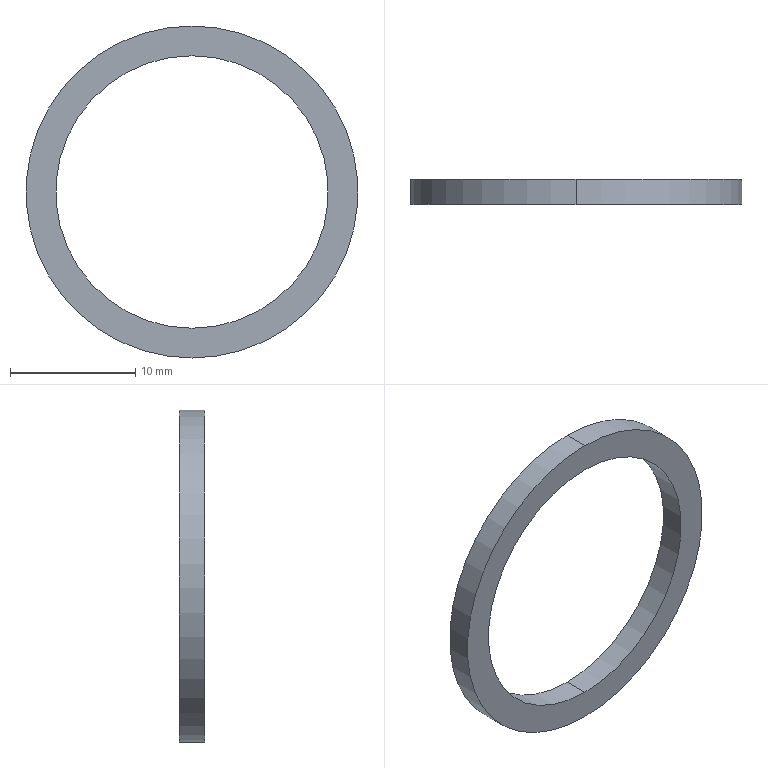Part | STEP file | 00649788_SCHEIBE_MKRT-23-16.5 | 1 solid | 6 faces | box 26.5 x 2 x 26.5 mm | volume 360.007 mm3 | cylinder 4 | plane 2 | commonest cylinder face diameters 21.75 x2 26.5 x2
STEP:
#1=CARTESIAN_POINT('',(0.,0.,0.));
#2=DIRECTION('',(0.,0.,1.));
#3=DIRECTION('',(1.,0.,0.));
#4=AXIS2_PLACEMENT_3D('',#1,#2,#3);
#5=CARTESIAN_POINT('',(0.,43.,10.875));
#6=VERTEX_POINT('',#5);
#7=CARTESIAN_POINT('',(0.,45.,10.875));
#8=VERTEX_POINT('',#7);
#9=CARTESIAN_POINT('',(0.,43.,10.875));
#10=DIRECTION('',(0.,1.,0.));
#11=VECTOR('',#10,1.);
#12=LINE('',#9,#11);
#13=CARTESIAN_POINT('',(0.,43.,0.));
#14=DIRECTION('',(0.,1.,0.));
#15=DIRECTION('',(0.,0.,1.));
#16=AXIS2_PLACEMENT_3D('',#13,#14,#15);
#17=CYLINDRICAL_SURFACE('',#16,10.875);
#18=CARTESIAN_POINT('',(6.283,0.));
#19=DIRECTION('',(0.,1.));
#20=VECTOR('',#19,1.);
#21=LINE('',#18,#20);
#22=(GEOMETRIC_REPRESENTATION_CONTEXT(2)PARAMETRIC_REPRESENTATION_CONTEXT()REPRESENTATION_CONTEXT('',''));
#23=DEFINITIONAL_REPRESENTATION('',(#21),#22);
#24=PCURVE('',#17,#23);
#25=CARTESIAN_POINT('',(0.,43.,0.));
#26=DIRECTION('',(0.,1.,0.));
#27=DIRECTION('',(0.,0.,1.));
#28=AXIS2_PLACEMENT_3D('',#25,#26,#27);
#29=CYLINDRICAL_SURFACE('',#28,10.875);
#30=CARTESIAN_POINT('',(0.,0.));
#31=DIRECTION('',(0.,1.));
#32=VECTOR('',#31,1.);
#33=LINE('',#30,#32);
#34=(GEOMETRIC_REPRESENTATION_CONTEXT(2)PARAMETRIC_REPRESENTATION_CONTEXT()REPRESENTATION_CONTEXT('',''));
#35=DEFINITIONAL_REPRESENTATION('',(#33),#34);
#36=PCURVE('',#29,#35);
#37=SURFACE_CURVE('',#12,(#24,#36),.PCURVE_S1.);
#38=EDGE_CURVE('',#6,#8,#37,.T.);
#39=ORIENTED_EDGE('',*,*,#38,.T.);
#40=CARTESIAN_POINT('',(0.,45.,-10.875));
#41=VERTEX_POINT('',#40);
#42=CARTESIAN_POINT('',(0.,45.,0.));
#43=DIRECTION('',(0.,-1.,0.));
#44=DIRECTION('',(0.,0.,1.));
#45=AXIS2_PLACEMENT_3D('',#42,#43,#44);
#46=CIRCLE('',#45,10.875);
#47=CARTESIAN_POINT('',(6.283,2.));
#48=DIRECTION('',(-1.,0.));
#49=VECTOR('',#48,1.);
#50=LINE('',#47,#49);
#51=(GEOMETRIC_REPRESENTATION_CONTEXT(2)PARAMETRIC_REPRESENTATION_CONTEXT()REPRESENTATION_CONTEXT('',''));
#52=DEFINITIONAL_REPRESENTATION('',(#50),#51);
#53=PCURVE('',#17,#52);
#54=CARTESIAN_POINT('',(40.672,45.,-24.269));
#55=DIRECTION('',(0.,1.,0.));
#56=DIRECTION('',(0.,0.,1.));
#57=AXIS2_PLACEMENT_3D('',#54,#55,#56);
#58=PLANE('',#57);
#59=CARTESIAN_POINT('',(35.144,-40.672));
#60=CARTESIAN_POINT('',(35.144,-59.508));
#61=CARTESIAN_POINT('',(18.831,-50.09));
#62=CARTESIAN_POINT('',(2.519,-40.672));
#63=CARTESIAN_POINT('',(18.831,-31.254));
#64=CARTESIAN_POINT('',(35.144,-21.836));
#65=CARTESIAN_POINT('',(35.144,-40.672));
#66=(BOUNDED_CURVE()B_SPLINE_CURVE(2,(#59,#60,#61,#62,#63,#64,#65),.UNSPECIFIED.,.T.,.F.)B_SPLINE_CURVE_WITH_KNOTS((1,2,2,2,2,1),(-2.094,0.,2.094,4.189,6.283,8.378),.UNSPECIFIED.)CURVE()GEOMETRIC_REPRESENTATION_ITEM()RATIONAL_B_SPLINE_CURVE((1.,0.5,1.,0.5,1.,0.5,1.))REPRESENTATION_ITEM(''));
#67=(GEOMETRIC_REPRESENTATION_CONTEXT(2)PARAMETRIC_REPRESENTATION_CONTEXT()REPRESENTATION_CONTEXT('',''));
#68=DEFINITIONAL_REPRESENTATION('',(#66),#67);
#69=PCURVE('',#58,#68);
#70=SURFACE_CURVE('',#46,(#53,#69),.PCURVE_S1.);
#71=EDGE_CURVE('',#8,#41,#70,.T.);
#72=ORIENTED_EDGE('',*,*,#71,.T.);
#73=CARTESIAN_POINT('',(0.,43.,-10.875));
#74=VERTEX_POINT('',#73);
#75=CARTESIAN_POINT('',(0.,43.,-10.875));
#76=DIRECTION('',(0.,1.,0.));
#77=VECTOR('',#76,1.);
#78=LINE('',#75,#77);
#79=CARTESIAN_POINT('',(3.142,0.));
#80=DIRECTION('',(0.,1.));
#81=VECTOR('',#80,1.);
#82=LINE('',#79,#81);
#83=(GEOMETRIC_REPRESENTATION_CONTEXT(2)PARAMETRIC_REPRESENTATION_CONTEXT()REPRESENTATION_CONTEXT('',''));
#84=DEFINITIONAL_REPRESENTATION('',(#82),#83);
#85=PCURVE('',#17,#84);
#86=CARTESIAN_POINT('',(3.142,0.));
#87=DIRECTION('',(0.,1.));
#88=VECTOR('',#87,1.);
#89=LINE('',#86,#88);
#90=(GEOMETRIC_REPRESENTATION_CONTEXT(2)PARAMETRIC_REPRESENTATION_CONTEXT()REPRESENTATION_CONTEXT('',''));
#91=DEFINITIONAL_REPRESENTATION('',(#89),#90);
#92=PCURVE('',#29,#91);
#93=SURFACE_CURVE('',#78,(#85,#92),.PCURVE_S1.);
#94=EDGE_CURVE('',#74,#41,#93,.T.);
#95=ORIENTED_EDGE('',*,*,#94,.F.);
#96=CARTESIAN_POINT('',(0.,43.,0.));
#97=DIRECTION('',(0.,-1.,0.));
#98=DIRECTION('',(0.,0.,1.));
#99=AXIS2_PLACEMENT_3D('',#96,#97,#98);
#100=CIRCLE('',#99,10.875);
#101=CARTESIAN_POINT('',(6.283,0.));
#102=DIRECTION('',(-1.,0.));
#103=VECTOR('',#102,1.);
#104=LINE('',#101,#103);
#105=(GEOMETRIC_REPRESENTATION_CONTEXT(2)PARAMETRIC_REPRESENTATION_CONTEXT()REPRESENTATION_CONTEXT('',''));
#106=DEFINITIONAL_REPRESENTATION('',(#104),#105);
#107=PCURVE('',#17,#106);
#108=CARTESIAN_POINT('',(40.672,43.,-24.269));
#109=DIRECTION('',(0.,1.,0.));
#110=DIRECTION('',(0.,0.,1.));
#111=AXIS2_PLACEMENT_3D('',#108,#109,#110);
#112=PLANE('',#111);
#113=CARTESIAN_POINT('',(35.144,-40.672));
#114=CARTESIAN_POINT('',(35.144,-59.508));
#115=CARTESIAN_POINT('',(18.831,-50.09));
#116=CARTESIAN_POINT('',(2.519,-40.672));
#117=CARTESIAN_POINT('',(18.831,-31.254));
#118=CARTESIAN_POINT('',(35.144,-21.836));
#119=CARTESIAN_POINT('',(35.144,-40.672));
#120=(BOUNDED_CURVE()B_SPLINE_CURVE(2,(#113,#114,#115,#116,#117,#118,#119),.UNSPECIFIED.,.T.,.F.)B_SPLINE_CURVE_WITH_KNOTS((1,2,2,2,2,1),(-2.094,0.,2.094,4.189,6.283,8.378),.UNSPECIFIED.)CURVE()GEOMETRIC_REPRESENTATION_ITEM()RATIONAL_B_SPLINE_CURVE((1.,0.5,1.,0.5,1.,0.5,1.))REPRESENTATION_ITEM(''));
#121=(GEOMETRIC_REPRESENTATION_CONTEXT(2)PARAMETRIC_REPRESENTATION_CONTEXT()REPRESENTATION_CONTEXT('',''));
#122=DEFINITIONAL_REPRESENTATION('',(#120),#121);
#123=PCURVE('',#112,#122);
#124=SURFACE_CURVE('',#100,(#107,#123),.PCURVE_S1.);
#125=EDGE_CURVE('',#6,#74,#124,.T.);
#126=ORIENTED_EDGE('',*,*,#125,.F.);
#127=EDGE_LOOP('',(#39,#72,#95,#126));
#128=FACE_BOUND('',#127,.F.);
#129=ADVANCED_FACE('',(#128),#17,.F.);
#130=CARTESIAN_POINT('',(0.,43.,13.25));
#131=VERTEX_POINT('',#130);
#132=CARTESIAN_POINT('',(0.,43.,-13.25));
#133=VERTEX_POINT('',#132);
#134=CARTESIAN_POINT('',(0.,43.,0.));
#135=DIRECTION('',(0.,1.,0.));
#136=DIRECTION('',(0.,0.,1.));
#137=AXIS2_PLACEMENT_3D('',#134,#135,#136);
#138=CIRCLE('',#137,13.25);
#139=CARTESIAN_POINT('',(0.,43.,0.));
#140=DIRECTION('',(0.,1.,0.));
#141=DIRECTION('',(0.,0.,1.));
#142=AXIS2_PLACEMENT_3D('',#139,#140,#141);
#143=CYLINDRICAL_SURFACE('',#142,13.25);
#144=CARTESIAN_POINT('',(0.,0.));
#145=DIRECTION('',(1.,0.));
#146=VECTOR('',#145,1.);
#147=LINE('',#144,#146);
#148=(GEOMETRIC_REPRESENTATION_CONTEXT(2)PARAMETRIC_REPRESENTATION_CONTEXT()REPRESENTATION_CONTEXT('',''));
#149=DEFINITIONAL_REPRESENTATION('',(#147),#148);
#150=PCURVE('',#143,#149);
#151=CARTESIAN_POINT('',(24.269,-40.672));
#152=DIRECTION('',(1.,0.));
#153=AXIS2_PLACEMENT_2D('',#151,#152);
#154=CIRCLE('',#153,13.25);
#155=(GEOMETRIC_REPRESENTATION_CONTEXT(2)PARAMETRIC_REPRESENTATION_CONTEXT()REPRESENTATION_CONTEXT('',''));
#156=DEFINITIONAL_REPRESENTATION('',(#154),#155);
#157=PCURVE('',#112,#156);
#158=SURFACE_CURVE('',#138,(#150,#157),.PCURVE_S1.);
#159=EDGE_CURVE('',#131,#133,#158,.T.);
#160=ORIENTED_EDGE('',*,*,#159,.T.);
#161=CARTESIAN_POINT('',(0.,45.,-13.25));
#162=VERTEX_POINT('',#161);
#163=CARTESIAN_POINT('',(0.,43.,-13.25));
#164=DIRECTION('',(0.,1.,0.));
#165=VECTOR('',#164,1.);
#166=LINE('',#163,#165);
#167=CARTESIAN_POINT('',(3.142,0.));
#168=DIRECTION('',(0.,1.));
#169=VECTOR('',#168,1.);
#170=LINE('',#167,#169);
#171=(GEOMETRIC_REPRESENTATION_CONTEXT(2)PARAMETRIC_REPRESENTATION_CONTEXT()REPRESENTATION_CONTEXT('',''));
#172=DEFINITIONAL_REPRESENTATION('',(#170),#171);
#173=PCURVE('',#143,#172);
#174=CARTESIAN_POINT('',(0.,43.,0.));
#175=DIRECTION('',(0.,1.,0.));
#176=DIRECTION('',(0.,0.,1.));
#177=AXIS2_PLACEMENT_3D('',#174,#175,#176);
#178=CYLINDRICAL_SURFACE('',#177,13.25);
#179=CARTESIAN_POINT('',(3.142,0.));
#180=DIRECTION('',(0.,1.));
#181=VECTOR('',#180,1.);
#182=LINE('',#179,#181);
#183=(GEOMETRIC_REPRESENTATION_CONTEXT(2)PARAMETRIC_REPRESENTATION_CONTEXT()REPRESENTATION_CONTEXT('',''));
#184=DEFINITIONAL_REPRESENTATION('',(#182),#183);
#185=PCURVE('',#178,#184);
#186=SURFACE_CURVE('',#166,(#173,#185),.PCURVE_S1.);
#187=EDGE_CURVE('',#133,#162,#186,.T.);
#188=ORIENTED_EDGE('',*,*,#187,.T.);
#189=CARTESIAN_POINT('',(0.,45.,13.25));
#190=VERTEX_POINT('',#189);
#191=CARTESIAN_POINT('',(0.,45.,0.));
#192=DIRECTION('',(0.,-1.,0.));
#193=DIRECTION('',(0.,0.,1.));
#194=AXIS2_PLACEMENT_3D('',#191,#192,#193);
#195=CIRCLE('',#194,13.25);
#196=CARTESIAN_POINT('',(6.283,2.));
#197=DIRECTION('',(-1.,0.));
#198=VECTOR('',#197,1.);
#199=LINE('',#196,#198);
#200=(GEOMETRIC_REPRESENTATION_CONTEXT(2)PARAMETRIC_REPRESENTATION_CONTEXT()REPRESENTATION_CONTEXT('',''));
#201=DEFINITIONAL_REPRESENTATION('',(#199),#200);
#202=PCURVE('',#143,#201);
#203=CARTESIAN_POINT('',(37.519,-40.672));
#204=CARTESIAN_POINT('',(37.519,-63.622));
#205=CARTESIAN_POINT('',(17.644,-52.147));
#206=CARTESIAN_POINT('',(-2.231,-40.672));
#207=CARTESIAN_POINT('',(17.644,-29.197));
#208=CARTESIAN_POINT('',(37.519,-17.722));
#209=CARTESIAN_POINT('',(37.519,-40.672));
#210=(BOUNDED_CURVE()B_SPLINE_CURVE(2,(#203,#204,#205,#206,#207,#208,#209),.UNSPECIFIED.,.T.,.F.)B_SPLINE_CURVE_WITH_KNOTS((1,2,2,2,2,1),(-2.094,0.,2.094,4.189,6.283,8.378),.UNSPECIFIED.)CURVE()GEOMETRIC_REPRESENTATION_ITEM()RATIONAL_B_SPLINE_CURVE((1.,0.5,1.,0.5,1.,0.5,1.))REPRESENTATION_ITEM(''));
#211=(GEOMETRIC_REPRESENTATION_CONTEXT(2)PARAMETRIC_REPRESENTATION_CONTEXT()REPRESENTATION_CONTEXT('',''));
#212=DEFINITIONAL_REPRESENTATION('',(#210),#211);
#213=PCURVE('',#58,#212);
#214=SURFACE_CURVE('',#195,(#202,#213),.PCURVE_S1.);
#215=EDGE_CURVE('',#162,#190,#214,.T.);
#216=ORIENTED_EDGE('',*,*,#215,.T.);
#217=CARTESIAN_POINT('',(0.,43.,13.25));
#218=DIRECTION('',(0.,1.,0.));
#219=VECTOR('',#218,1.);
#220=LINE('',#217,#219);
#221=CARTESIAN_POINT('',(0.,0.));
#222=DIRECTION('',(0.,1.));
#223=VECTOR('',#222,1.);
#224=LINE('',#221,#223);
#225=(GEOMETRIC_REPRESENTATION_CONTEXT(2)PARAMETRIC_REPRESENTATION_CONTEXT()REPRESENTATION_CONTEXT('',''));
#226=DEFINITIONAL_REPRESENTATION('',(#224),#225);
#227=PCURVE('',#143,#226);
#228=CARTESIAN_POINT('',(6.283,0.));
#229=DIRECTION('',(0.,1.));
#230=VECTOR('',#229,1.);
#231=LINE('',#228,#230);
#232=(GEOMETRIC_REPRESENTATION_CONTEXT(2)PARAMETRIC_REPRESENTATION_CONTEXT()REPRESENTATION_CONTEXT('',''));
#233=DEFINITIONAL_REPRESENTATION('',(#231),#232);
#234=PCURVE('',#178,#233);
#235=SURFACE_CURVE('',#220,(#227,#234),.PCURVE_S1.);
#236=EDGE_CURVE('',#131,#190,#235,.T.);
#237=ORIENTED_EDGE('',*,*,#236,.F.);
#238=EDGE_LOOP('',(#160,#188,#216,#237));
#239=FACE_BOUND('',#238,.T.);
#240=ADVANCED_FACE('',(#239),#143,.T.);
#241=ORIENTED_EDGE('',*,*,#71,.T.);
#242=CARTESIAN_POINT('',(0.,45.,0.));
#243=DIRECTION('',(0.,-1.,0.));
#244=DIRECTION('',(0.,0.,1.));
#245=AXIS2_PLACEMENT_3D('',#242,#243,#244);
#246=CIRCLE('',#245,10.875);
#247=CARTESIAN_POINT('',(35.144,-40.672));
#248=CARTESIAN_POINT('',(35.144,-59.508));
#249=CARTESIAN_POINT('',(18.831,-50.09));
#250=CARTESIAN_POINT('',(2.519,-40.672));
#251=CARTESIAN_POINT('',(18.831,-31.254));
#252=CARTESIAN_POINT('',(35.144,-21.836));
#253=CARTESIAN_POINT('',(35.144,-40.672));
#254=(BOUNDED_CURVE()B_SPLINE_CURVE(2,(#247,#248,#249,#250,#251,#252,#253),.UNSPECIFIED.,.T.,.F.)B_SPLINE_CURVE_WITH_KNOTS((1,2,2,2,2,1),(-2.094,0.,2.094,4.189,6.283,8.378),.UNSPECIFIED.)CURVE()GEOMETRIC_REPRESENTATION_ITEM()RATIONAL_B_SPLINE_CURVE((1.,0.5,1.,0.5,1.,0.5,1.))REPRESENTATION_ITEM(''));
#255=(GEOMETRIC_REPRESENTATION_CONTEXT(2)PARAMETRIC_REPRESENTATION_CONTEXT()REPRESENTATION_CONTEXT('',''));
#256=DEFINITIONAL_REPRESENTATION('',(#254),#255);
#257=PCURVE('',#58,#256);
#258=CARTESIAN_POINT('',(6.283,2.));
#259=DIRECTION('',(-1.,0.));
#260=VECTOR('',#259,1.);
#261=LINE('',#258,#260);
#262=(GEOMETRIC_REPRESENTATION_CONTEXT(2)PARAMETRIC_REPRESENTATION_CONTEXT()REPRESENTATION_CONTEXT('',''));
#263=DEFINITIONAL_REPRESENTATION('',(#261),#262);
#264=PCURVE('',#29,#263);
#265=SURFACE_CURVE('',#246,(#257,#264),.PCURVE_S1.);
#266=EDGE_CURVE('',#41,#8,#265,.T.);
#267=ORIENTED_EDGE('',*,*,#266,.T.);
#268=EDGE_LOOP('',(#241,#267));
#269=FACE_BOUND('',#268,.T.);
#270=CARTESIAN_POINT('',(0.,45.,0.));
#271=DIRECTION('',(0.,-1.,0.));
#272=DIRECTION('',(0.,0.,1.));
#273=AXIS2_PLACEMENT_3D('',#270,#271,#272);
#274=CIRCLE('',#273,13.25);
#275=CARTESIAN_POINT('',(37.519,-40.672));
#276=CARTESIAN_POINT('',(37.519,-63.622));
#277=CARTESIAN_POINT('',(17.644,-52.147));
#278=CARTESIAN_POINT('',(-2.231,-40.672));
#279=CARTESIAN_POINT('',(17.644,-29.197));
#280=CARTESIAN_POINT('',(37.519,-17.722));
#281=CARTESIAN_POINT('',(37.519,-40.672));
#282=(BOUNDED_CURVE()B_SPLINE_CURVE(2,(#275,#276,#277,#278,#279,#280,#281),.UNSPECIFIED.,.T.,.F.)B_SPLINE_CURVE_WITH_KNOTS((1,2,2,2,2,1),(-2.094,0.,2.094,4.189,6.283,8.378),.UNSPECIFIED.)CURVE()GEOMETRIC_REPRESENTATION_ITEM()RATIONAL_B_SPLINE_CURVE((1.,0.5,1.,0.5,1.,0.5,1.))REPRESENTATION_ITEM(''));
#283=(GEOMETRIC_REPRESENTATION_CONTEXT(2)PARAMETRIC_REPRESENTATION_CONTEXT()REPRESENTATION_CONTEXT('',''));
#284=DEFINITIONAL_REPRESENTATION('',(#282),#283);
#285=PCURVE('',#58,#284);
#286=CARTESIAN_POINT('',(6.283,2.));
#287=DIRECTION('',(-1.,0.));
#288=VECTOR('',#287,1.);
#289=LINE('',#286,#288);
#290=(GEOMETRIC_REPRESENTATION_CONTEXT(2)PARAMETRIC_REPRESENTATION_CONTEXT()REPRESENTATION_CONTEXT('',''));
#291=DEFINITIONAL_REPRESENTATION('',(#289),#290);
#292=PCURVE('',#178,#291);
#293=SURFACE_CURVE('',#274,(#285,#292),.PCURVE_S1.);
#294=EDGE_CURVE('',#190,#162,#293,.T.);
#295=ORIENTED_EDGE('',*,*,#294,.F.);
#296=ORIENTED_EDGE('',*,*,#215,.F.);
#297=EDGE_LOOP('',(#295,#296));
#298=FACE_BOUND('',#297,.T.);
#299=ADVANCED_FACE('',(#269,#298),#58,.T.);
#300=ORIENTED_EDGE('',*,*,#187,.F.);
#301=CARTESIAN_POINT('',(0.,43.,0.));
#302=DIRECTION('',(0.,1.,0.));
#303=DIRECTION('',(0.,0.,1.));
#304=AXIS2_PLACEMENT_3D('',#301,#302,#303);
#305=CIRCLE('',#304,13.25);
#306=CARTESIAN_POINT('',(0.,0.));
#307=DIRECTION('',(1.,0.));
#308=VECTOR('',#307,1.);
#309=LINE('',#306,#308);
#310=(GEOMETRIC_REPRESENTATION_CONTEXT(2)PARAMETRIC_REPRESENTATION_CONTEXT()REPRESENTATION_CONTEXT('',''));
#311=DEFINITIONAL_REPRESENTATION('',(#309),#310);
#312=PCURVE('',#178,#311);
#313=CARTESIAN_POINT('',(24.269,-40.672));
#314=DIRECTION('',(1.,0.));
#315=AXIS2_PLACEMENT_2D('',#313,#314);
#316=CIRCLE('',#315,13.25);
#317=(GEOMETRIC_REPRESENTATION_CONTEXT(2)PARAMETRIC_REPRESENTATION_CONTEXT()REPRESENTATION_CONTEXT('',''));
#318=DEFINITIONAL_REPRESENTATION('',(#316),#317);
#319=PCURVE('',#112,#318);
#320=SURFACE_CURVE('',#305,(#312,#319),.PCURVE_S1.);
#321=EDGE_CURVE('',#133,#131,#320,.T.);
#322=ORIENTED_EDGE('',*,*,#321,.T.);
#323=ORIENTED_EDGE('',*,*,#236,.T.);
#324=ORIENTED_EDGE('',*,*,#294,.T.);
#325=EDGE_LOOP('',(#300,#322,#323,#324));
#326=FACE_BOUND('',#325,.T.);
#327=ADVANCED_FACE('',(#326),#178,.T.);
#328=ORIENTED_EDGE('',*,*,#266,.T.);
#329=ORIENTED_EDGE('',*,*,#38,.F.);
#330=CARTESIAN_POINT('',(0.,43.,0.));
#331=DIRECTION('',(0.,-1.,0.));
#332=DIRECTION('',(0.,0.,1.));
#333=AXIS2_PLACEMENT_3D('',#330,#331,#332);
#334=CIRCLE('',#333,10.875);
#335=CARTESIAN_POINT('',(6.283,0.));
#336=DIRECTION('',(-1.,0.));
#337=VECTOR('',#336,1.);
#338=LINE('',#335,#337);
#339=(GEOMETRIC_REPRESENTATION_CONTEXT(2)PARAMETRIC_REPRESENTATION_CONTEXT()REPRESENTATION_CONTEXT('',''));
#340=DEFINITIONAL_REPRESENTATION('',(#338),#339);
#341=PCURVE('',#29,#340);
#342=CARTESIAN_POINT('',(35.144,-40.672));
#343=CARTESIAN_POINT('',(35.144,-59.508));
#344=CARTESIAN_POINT('',(18.831,-50.09));
#345=CARTESIAN_POINT('',(2.519,-40.672));
#346=CARTESIAN_POINT('',(18.831,-31.254));
#347=CARTESIAN_POINT('',(35.144,-21.836));
#348=CARTESIAN_POINT('',(35.144,-40.672));
#349=(BOUNDED_CURVE()B_SPLINE_CURVE(2,(#342,#343,#344,#345,#346,#347,#348),.UNSPECIFIED.,.T.,.F.)B_SPLINE_CURVE_WITH_KNOTS((1,2,2,2,2,1),(-2.094,0.,2.094,4.189,6.283,8.378),.UNSPECIFIED.)CURVE()GEOMETRIC_REPRESENTATION_ITEM()RATIONAL_B_SPLINE_CURVE((1.,0.5,1.,0.5,1.,0.5,1.))REPRESENTATION_ITEM(''));
#350=(GEOMETRIC_REPRESENTATION_CONTEXT(2)PARAMETRIC_REPRESENTATION_CONTEXT()REPRESENTATION_CONTEXT('',''));
#351=DEFINITIONAL_REPRESENTATION('',(#349),#350);
#352=PCURVE('',#112,#351);
#353=SURFACE_CURVE('',#334,(#341,#352),.PCURVE_S1.);
#354=EDGE_CURVE('',#74,#6,#353,.T.);
#355=ORIENTED_EDGE('',*,*,#354,.F.);
#356=ORIENTED_EDGE('',*,*,#94,.T.);
#357=EDGE_LOOP('',(#328,#329,#355,#356));
#358=FACE_BOUND('',#357,.F.);
#359=ADVANCED_FACE('',(#358),#29,.F.);
#360=ORIENTED_EDGE('',*,*,#125,.F.);
#361=ORIENTED_EDGE('',*,*,#354,.F.);
#362=EDGE_LOOP('',(#360,#361));
#363=FACE_BOUND('',#362,.T.);
#364=ORIENTED_EDGE('',*,*,#159,.F.);
#365=ORIENTED_EDGE('',*,*,#321,.F.);
#366=EDGE_LOOP('',(#364,#365));
#367=FACE_BOUND('',#366,.T.);
#368=ADVANCED_FACE('',(#363,#367),#112,.F.);
#369=CLOSED_SHELL('',(#129,#240,#299,#327,#359,#368));
#370=MANIFOLD_SOLID_BREP('',#369);
#371=(LENGTH_UNIT()NAMED_UNIT(*)SI_UNIT(.MILLI.,.METRE.));
#372=UNCERTAINTY_MEASURE_WITH_UNIT(LENGTH_MEASURE(0.0000001),#371,'','');
#373=(NAMED_UNIT(*)PLANE_ANGLE_UNIT()SI_UNIT($,.RADIAN.));
#374=(NAMED_UNIT(*)SI_UNIT($,.STERADIAN.)SOLID_ANGLE_UNIT());
#375=(GEOMETRIC_REPRESENTATION_CONTEXT(3)GLOBAL_UNCERTAINTY_ASSIGNED_CONTEXT((#372))GLOBAL_UNIT_ASSIGNED_CONTEXT((#371,#373,#374))REPRESENTATION_CONTEXT('',''));
#376=ADVANCED_BREP_SHAPE_REPRESENTATION('',(#4,#370),#375);